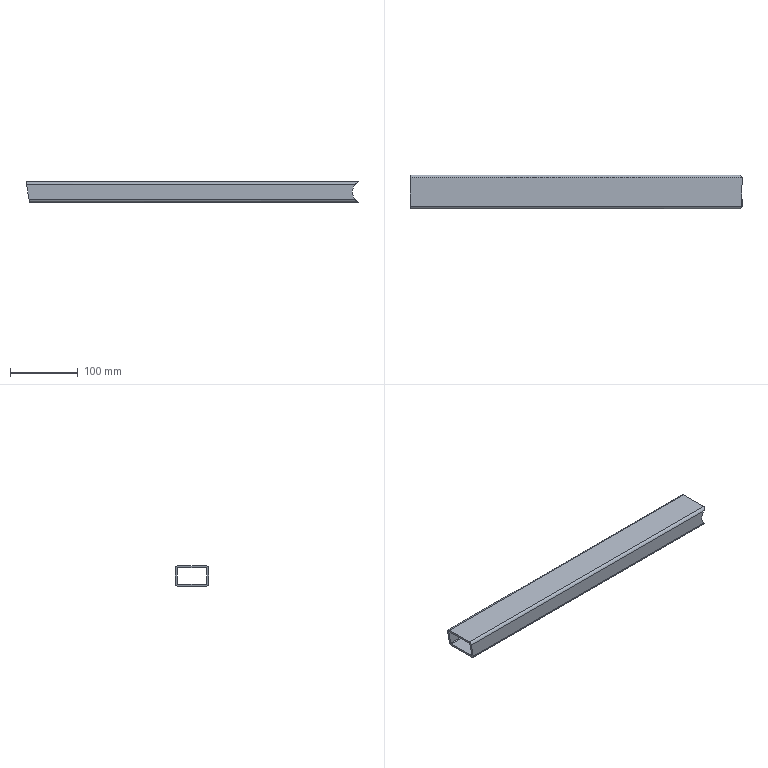Part | SolidWorks | features ICE 2, WeldMemberFeat 1, WeldmentFeature 1 | 1 solid | 18 faces | box 490.986 x 50 x 30 mm | volume 208931 mm3 | cylinder 9 | plane 9 | commonest cylinder face diameters 2 x4 8 x4 35 x1
STEP:
#1=CARTESIAN_POINT('',(-499.295,-25.,11.));
#2=VERTEX_POINT('',#1);
#3=CARTESIAN_POINT('',(-13.611,-25.,11.));
#4=VERTEX_POINT('',#3);
#5=CARTESIAN_POINT('',(-600.,-25.,11.));
#6=DIRECTION('',(1.,0.,0.));
#7=VECTOR('',#6,1000.);
#8=LINE('',#5,#7);
#9=EDGE_CURVE('',#2,#4,#8,.T.);
#10=ORIENTED_EDGE('',*,*,#9,.T.);
#11=CARTESIAN_POINT('',(-9.014,-21.,15.));
#12=VERTEX_POINT('',#11);
#13=CARTESIAN_POINT('',(-13.611,-25.,11.));
#14=CARTESIAN_POINT('',(-13.193,-25.,11.517));
#15=CARTESIAN_POINT('',(-12.756,-24.903,11.998));
#16=CARTESIAN_POINT('',(-11.846,-24.554,12.897));
#17=CARTESIAN_POINT('',(-11.388,-24.308,13.3));
#18=CARTESIAN_POINT('',(-10.713,-23.827,13.84));
#19=CARTESIAN_POINT('',(-10.49,-23.646,14.01));
#20=CARTESIAN_POINT('',(-10.065,-23.248,14.318));
#21=CARTESIAN_POINT('',(-9.861,-23.028,14.459));
#22=CARTESIAN_POINT('',(-9.491,-22.533,14.705));
#23=CARTESIAN_POINT('',(-9.328,-22.264,14.808));
#24=CARTESIAN_POINT('',(-9.146,-21.812,14.92));
#25=CARTESIAN_POINT('',(-9.098,-21.656,14.949));
#26=CARTESIAN_POINT('',(-9.032,-21.335,14.989));
#27=CARTESIAN_POINT('',(-9.014,-21.167,15.));
#28=CARTESIAN_POINT('',(-9.014,-21.,15.));
#29=B_SPLINE_CURVE_WITH_KNOTS('',3,(#13,#14,#15,#16,#17,#18,#19,#20,#21,#22,#23,#24,#25,#26,#27,#28),.UNSPECIFIED.,.F.,.F.,(4,2,2,2,2,2,2,4),(0.,0.001971,0.003942,0.004927,0.005913,0.006898,0.007391,0.007884),.UNSPECIFIED.);
#30=EDGE_CURVE('',#4,#12,#29,.T.);
#31=ORIENTED_EDGE('',*,*,#30,.T.);
#32=CARTESIAN_POINT('',(-500.,-21.,15.));
#33=VERTEX_POINT('',#32);
#34=CARTESIAN_POINT('',(-600.,-21.,15.));
#35=DIRECTION('',(1.,0.,0.));
#36=VECTOR('',#35,1000.);
#37=LINE('',#34,#36);
#38=EDGE_CURVE('',#33,#12,#37,.T.);
#39=ORIENTED_EDGE('',*,*,#38,.F.);
#40=CARTESIAN_POINT('',(-500.,-21.,15.));
#41=CARTESIAN_POINT('',(-500.,-23.343,15.));
#42=CARTESIAN_POINT('',(-499.708,-25.,13.343));
#43=CARTESIAN_POINT('',(-499.295,-25.,11.));
#44=(BOUNDED_CURVE()B_SPLINE_CURVE(3,(#40,#41,#42,#43),.UNSPECIFIED.,.F.,.F.)B_SPLINE_CURVE_WITH_KNOTS((4,4),(3.142,4.712),.UNSPECIFIED.)CURVE()GEOMETRIC_REPRESENTATION_ITEM()RATIONAL_B_SPLINE_CURVE((1.,0.8047,0.8047,1.))REPRESENTATION_ITEM(''));
#45=EDGE_CURVE('',#33,#2,#44,.T.);
#46=ORIENTED_EDGE('',*,*,#45,.T.);
#47=EDGE_LOOP('',(#10,#31,#39,#46));
#48=FACE_OUTER_BOUND('',#47,.T.);
#49=CARTESIAN_POINT('',(-600.,-21.,11.));
#50=DIRECTION('',(1.,0.,0.));
#51=DIRECTION('',(0.,1.,0.));
#52=AXIS2_PLACEMENT_3D('',#49,#50,#51);
#53=CYLINDRICAL_SURFACE('',#52,4.);
#54=ADVANCED_FACE('',(#48),#53,.T.);
#55=ORIENTED_EDGE('',*,*,#38,.T.);
#56=CARTESIAN_POINT('',(-9.014,21.,15.));
#57=VERTEX_POINT('',#56);
#58=CARTESIAN_POINT('',(-9.014,88.,15.));
#59=DIRECTION('',(0.,1.,0.));
#60=VECTOR('',#59,1000.);
#61=LINE('',#58,#60);
#62=EDGE_CURVE('',#12,#57,#61,.T.);
#63=ORIENTED_EDGE('',*,*,#62,.T.);
#64=CARTESIAN_POINT('',(-500.,21.,15.));
#65=VERTEX_POINT('',#64);
#66=CARTESIAN_POINT('',(-600.,21.,15.));
#67=DIRECTION('',(1.,0.,0.));
#68=VECTOR('',#67,1000.);
#69=LINE('',#66,#68);
#70=EDGE_CURVE('',#65,#57,#69,.T.);
#71=ORIENTED_EDGE('',*,*,#70,.F.);
#72=CARTESIAN_POINT('',(-500.,88.,15.));
#73=DIRECTION('',(0.,-1.,0.));
#74=VECTOR('',#73,1000.);
#75=LINE('',#72,#74);
#76=EDGE_CURVE('',#65,#33,#75,.T.);
#77=ORIENTED_EDGE('',*,*,#76,.T.);
#78=EDGE_LOOP('',(#55,#63,#71,#77));
#79=FACE_OUTER_BOUND('',#78,.T.);
#80=CARTESIAN_POINT('',(-600.,-21.,15.));
#81=DIRECTION('',(0.,0.,-1.));
#82=DIRECTION('',(-1.,0.,0.));
#83=AXIS2_PLACEMENT_3D('',#80,#81,#82);
#84=PLANE('',#83);
#85=ADVANCED_FACE('',(#79),#84,.F.);
#86=ORIENTED_EDGE('',*,*,#70,.T.);
#87=CARTESIAN_POINT('',(-13.611,25.,11.));
#88=VERTEX_POINT('',#87);
#89=CARTESIAN_POINT('',(-9.014,21.,15.));
#90=CARTESIAN_POINT('',(-9.014,21.168,15.));
#91=CARTESIAN_POINT('',(-9.031,21.332,14.989));
#92=CARTESIAN_POINT('',(-9.098,21.654,14.949));
#93=CARTESIAN_POINT('',(-9.147,21.813,14.92));
#94=CARTESIAN_POINT('',(-9.267,22.113,14.845));
#95=CARTESIAN_POINT('',(-9.338,22.255,14.801));
#96=CARTESIAN_POINT('',(-9.497,22.528,14.699));
#97=CARTESIAN_POINT('',(-9.585,22.659,14.642));
#98=CARTESIAN_POINT('',(-9.862,23.028,14.459));
#99=CARTESIAN_POINT('',(-10.064,23.247,14.319));
#100=CARTESIAN_POINT('',(-10.49,23.647,14.01));
#101=CARTESIAN_POINT('',(-10.714,23.827,13.84));
#102=CARTESIAN_POINT('',(-11.163,24.147,13.481));
#103=CARTESIAN_POINT('',(-11.389,24.288,13.29));
#104=CARTESIAN_POINT('',(-11.844,24.535,12.887));
#105=CARTESIAN_POINT('',(-12.074,24.642,12.672));
#106=CARTESIAN_POINT('',(-12.755,24.903,11.998));
#107=CARTESIAN_POINT('',(-13.192,25.,11.518));
#108=CARTESIAN_POINT('',(-13.611,25.,11.));
#109=B_SPLINE_CURVE_WITH_KNOTS('',3,(#89,#90,#91,#92,#93,#94,#95,#96,#97,#98,#99,#100,#101,#102,#103,#104,#105,#106,#107,#108),.UNSPECIFIED.,.F.,.F.,(4,2,2,2,2,2,2,2,2,4),(0.,0.0004959,0.0009918,0.001488,0.001984,0.002975,0.003967,0.004959,0.005951,0.007934),.UNSPECIFIED.);
#110=EDGE_CURVE('',#57,#88,#109,.T.);
#111=ORIENTED_EDGE('',*,*,#110,.T.);
#112=CARTESIAN_POINT('',(-499.295,25.,11.));
#113=VERTEX_POINT('',#112);
#114=CARTESIAN_POINT('',(-600.,25.,11.));
#115=DIRECTION('',(1.,0.,0.));
#116=VECTOR('',#115,1000.);
#117=LINE('',#114,#116);
#118=EDGE_CURVE('',#113,#88,#117,.T.);
#119=ORIENTED_EDGE('',*,*,#118,.F.);
#120=CARTESIAN_POINT('',(-499.295,25.,11.));
#121=CARTESIAN_POINT('',(-499.708,25.,13.343));
#122=CARTESIAN_POINT('',(-500.,23.343,15.));
#123=CARTESIAN_POINT('',(-500.,21.,15.));
#124=(BOUNDED_CURVE()B_SPLINE_CURVE(3,(#120,#121,#122,#123),.UNSPECIFIED.,.F.,.F.)B_SPLINE_CURVE_WITH_KNOTS((4,4),(1.571,3.142),.UNSPECIFIED.)CURVE()GEOMETRIC_REPRESENTATION_ITEM()RATIONAL_B_SPLINE_CURVE((1.,0.8047,0.8047,1.))REPRESENTATION_ITEM(''));
#125=EDGE_CURVE('',#113,#65,#124,.T.);
#126=ORIENTED_EDGE('',*,*,#125,.T.);
#127=EDGE_LOOP('',(#86,#111,#119,#126));
#128=FACE_OUTER_BOUND('',#127,.T.);
#129=CARTESIAN_POINT('',(-600.,21.,11.));
#130=DIRECTION('',(1.,0.,0.));
#131=DIRECTION('',(0.,1.,0.));
#132=AXIS2_PLACEMENT_3D('',#129,#130,#131);
#133=CYLINDRICAL_SURFACE('',#132,4.);
#134=ADVANCED_FACE('',(#128),#133,.T.);
#135=ORIENTED_EDGE('',*,*,#118,.T.);
#136=CARTESIAN_POINT('',(-13.611,25.,-11.));
#137=VERTEX_POINT('',#136);
#138=CARTESIAN_POINT('',(0.,25.,0.));
#139=DIRECTION('',(0.,-1.,0.));
#140=DIRECTION('',(1.,0.,0.));
#141=AXIS2_PLACEMENT_3D('',#138,#139,#140);
#142=CIRCLE('',#141,17.5);
#143=EDGE_CURVE('',#88,#137,#142,.T.);
#144=ORIENTED_EDGE('',*,*,#143,.T.);
#145=CARTESIAN_POINT('',(-495.415,25.,-11.));
#146=VERTEX_POINT('',#145);
#147=CARTESIAN_POINT('',(-600.,25.,-11.));
#148=DIRECTION('',(1.,0.,0.));
#149=VECTOR('',#148,1000.);
#150=LINE('',#147,#149);
#151=EDGE_CURVE('',#146,#137,#150,.T.);
#152=ORIENTED_EDGE('',*,*,#151,.F.);
#153=CARTESIAN_POINT('',(-498.569,25.,6.885));
#154=DIRECTION('',(-0.1736,0.,0.9848));
#155=VECTOR('',#154,1000.);
#156=LINE('',#153,#155);
#157=EDGE_CURVE('',#146,#113,#156,.T.);
#158=ORIENTED_EDGE('',*,*,#157,.T.);
#159=EDGE_LOOP('',(#135,#144,#152,#158));
#160=FACE_OUTER_BOUND('',#159,.T.);
#161=CARTESIAN_POINT('',(-600.,25.,-11.));
#162=DIRECTION('',(0.,-1.,0.));
#163=DIRECTION('',(1.,0.,0.));
#164=AXIS2_PLACEMENT_3D('',#161,#162,#163);
#165=PLANE('',#164);
#166=ADVANCED_FACE('',(#160),#165,.F.);
#167=ORIENTED_EDGE('',*,*,#151,.T.);
#168=CARTESIAN_POINT('',(-9.014,21.,-15.));
#169=VERTEX_POINT('',#168);
#170=CARTESIAN_POINT('',(-13.611,25.,-11.));
#171=CARTESIAN_POINT('',(-13.193,25.,-11.517));
#172=CARTESIAN_POINT('',(-12.756,24.903,-11.998));
#173=CARTESIAN_POINT('',(-11.846,24.554,-12.897));
#174=CARTESIAN_POINT('',(-11.388,24.308,-13.3));
#175=CARTESIAN_POINT('',(-10.713,23.827,-13.84));
#176=CARTESIAN_POINT('',(-10.49,23.646,-14.01));
#177=CARTESIAN_POINT('',(-10.065,23.248,-14.318));
#178=CARTESIAN_POINT('',(-9.861,23.028,-14.459));
#179=CARTESIAN_POINT('',(-9.491,22.533,-14.705));
#180=CARTESIAN_POINT('',(-9.328,22.264,-14.808));
#181=CARTESIAN_POINT('',(-9.146,21.812,-14.92));
#182=CARTESIAN_POINT('',(-9.098,21.656,-14.949));
#183=CARTESIAN_POINT('',(-9.032,21.335,-14.989));
#184=CARTESIAN_POINT('',(-9.014,21.167,-15.));
#185=CARTESIAN_POINT('',(-9.014,21.,-15.));
#186=B_SPLINE_CURVE_WITH_KNOTS('',3,(#170,#171,#172,#173,#174,#175,#176,#177,#178,#179,#180,#181,#182,#183,#184,#185),.UNSPECIFIED.,.F.,.F.,(4,2,2,2,2,2,2,4),(0.,0.001971,0.003942,0.004927,0.005913,0.006898,0.007391,0.007884),.UNSPECIFIED.);
#187=EDGE_CURVE('',#137,#169,#186,.T.);
#188=ORIENTED_EDGE('',*,*,#187,.T.);
#189=CARTESIAN_POINT('',(-494.71,21.,-15.));
#190=VERTEX_POINT('',#189);
#191=CARTESIAN_POINT('',(-600.,21.,-15.));
#192=DIRECTION('',(1.,0.,0.));
#193=VECTOR('',#192,1000.);
#194=LINE('',#191,#193);
#195=EDGE_CURVE('',#190,#169,#194,.T.);
#196=ORIENTED_EDGE('',*,*,#195,.F.);
#197=CARTESIAN_POINT('',(-494.71,21.,-15.));
#198=CARTESIAN_POINT('',(-494.71,23.343,-15.));
#199=CARTESIAN_POINT('',(-495.002,25.,-13.343));
#200=CARTESIAN_POINT('',(-495.415,25.,-11.));
#201=(BOUNDED_CURVE()B_SPLINE_CURVE(3,(#197,#198,#199,#200),.UNSPECIFIED.,.F.,.F.)B_SPLINE_CURVE_WITH_KNOTS((4,4),(0.,1.571),.UNSPECIFIED.)CURVE()GEOMETRIC_REPRESENTATION_ITEM()RATIONAL_B_SPLINE_CURVE((1.,0.8047,0.8047,1.))REPRESENTATION_ITEM(''));
#202=EDGE_CURVE('',#190,#146,#201,.T.);
#203=ORIENTED_EDGE('',*,*,#202,.T.);
#204=EDGE_LOOP('',(#167,#188,#196,#203));
#205=FACE_OUTER_BOUND('',#204,.T.);
#206=CARTESIAN_POINT('',(-600.,21.,-11.));
#207=DIRECTION('',(1.,0.,0.));
#208=DIRECTION('',(0.,1.,0.));
#209=AXIS2_PLACEMENT_3D('',#206,#207,#208);
#210=CYLINDRICAL_SURFACE('',#209,4.);
#211=ADVANCED_FACE('',(#205),#210,.T.);
#212=ORIENTED_EDGE('',*,*,#195,.T.);
#213=CARTESIAN_POINT('',(-9.014,-21.,-15.));
#214=VERTEX_POINT('',#213);
#215=CARTESIAN_POINT('',(-9.014,88.,-15.));
#216=DIRECTION('',(0.,-1.,0.));
#217=VECTOR('',#216,1000.);
#218=LINE('',#215,#217);
#219=EDGE_CURVE('',#169,#214,#218,.T.);
#220=ORIENTED_EDGE('',*,*,#219,.T.);
#221=CARTESIAN_POINT('',(-494.71,-21.,-15.));
#222=VERTEX_POINT('',#221);
#223=CARTESIAN_POINT('',(-600.,-21.,-15.));
#224=DIRECTION('',(1.,0.,0.));
#225=VECTOR('',#224,1000.);
#226=LINE('',#223,#225);
#227=EDGE_CURVE('',#222,#214,#226,.T.);
#228=ORIENTED_EDGE('',*,*,#227,.F.);
#229=CARTESIAN_POINT('',(-494.71,88.,-15.));
#230=DIRECTION('',(0.,-1.,0.));
#231=VECTOR('',#230,1000.);
#232=LINE('',#229,#231);
#233=EDGE_CURVE('',#190,#222,#232,.T.);
#234=ORIENTED_EDGE('',*,*,#233,.F.);
#235=EDGE_LOOP('',(#212,#220,#228,#234));
#236=FACE_OUTER_BOUND('',#235,.T.);
#237=CARTESIAN_POINT('',(-600.,21.,-15.));
#238=DIRECTION('',(0.,0.,1.));
#239=DIRECTION('',(1.,0.,0.));
#240=AXIS2_PLACEMENT_3D('',#237,#238,#239);
#241=PLANE('',#240);
#242=ADVANCED_FACE('',(#236),#241,.F.);
#243=ORIENTED_EDGE('',*,*,#227,.T.);
#244=CARTESIAN_POINT('',(-13.611,-25.,-11.));
#245=VERTEX_POINT('',#244);
#246=CARTESIAN_POINT('',(-9.014,-21.,-15.));
#247=CARTESIAN_POINT('',(-9.014,-21.168,-15.));
#248=CARTESIAN_POINT('',(-9.031,-21.332,-14.989));
#249=CARTESIAN_POINT('',(-9.098,-21.654,-14.949));
#250=CARTESIAN_POINT('',(-9.147,-21.813,-14.92));
#251=CARTESIAN_POINT('',(-9.267,-22.113,-14.845));
#252=CARTESIAN_POINT('',(-9.338,-22.255,-14.801));
#253=CARTESIAN_POINT('',(-9.497,-22.528,-14.699));
#254=CARTESIAN_POINT('',(-9.585,-22.659,-14.642));
#255=CARTESIAN_POINT('',(-9.862,-23.028,-14.459));
#256=CARTESIAN_POINT('',(-10.064,-23.247,-14.319));
#257=CARTESIAN_POINT('',(-10.49,-23.647,-14.01));
#258=CARTESIAN_POINT('',(-10.714,-23.827,-13.84));
#259=CARTESIAN_POINT('',(-11.163,-24.147,-13.481));
#260=CARTESIAN_POINT('',(-11.389,-24.288,-13.29));
#261=CARTESIAN_POINT('',(-11.844,-24.535,-12.887));
#262=CARTESIAN_POINT('',(-12.074,-24.642,-12.672));
#263=CARTESIAN_POINT('',(-12.755,-24.903,-11.998));
#264=CARTESIAN_POINT('',(-13.192,-25.,-11.518));
#265=CARTESIAN_POINT('',(-13.611,-25.,-11.));
#266=B_SPLINE_CURVE_WITH_KNOTS('',3,(#246,#247,#248,#249,#250,#251,#252,#253,#254,#255,#256,#257,#258,#259,#260,#261,#262,#263,#264,#265),.UNSPECIFIED.,.F.,.F.,(4,2,2,2,2,2,2,2,2,4),(0.,0.0004959,0.0009918,0.001488,0.001984,0.002975,0.003967,0.004959,0.005951,0.007934),.UNSPECIFIED.);
#267=EDGE_CURVE('',#214,#245,#266,.T.);
#268=ORIENTED_EDGE('',*,*,#267,.T.);
#269=CARTESIAN_POINT('',(-495.415,-25.,-11.));
#270=VERTEX_POINT('',#269);
#271=CARTESIAN_POINT('',(-600.,-25.,-11.));
#272=DIRECTION('',(1.,0.,0.));
#273=VECTOR('',#272,1000.);
#274=LINE('',#271,#273);
#275=EDGE_CURVE('',#270,#245,#274,.T.);
#276=ORIENTED_EDGE('',*,*,#275,.F.);
#277=CARTESIAN_POINT('',(-495.415,-25.,-11.));
#278=CARTESIAN_POINT('',(-495.002,-25.,-13.343));
#279=CARTESIAN_POINT('',(-494.71,-23.343,-15.));
#280=CARTESIAN_POINT('',(-494.71,-21.,-15.));
#281=(BOUNDED_CURVE()B_SPLINE_CURVE(3,(#277,#278,#279,#280),.UNSPECIFIED.,.F.,.F.)B_SPLINE_CURVE_WITH_KNOTS((4,4),(4.712,6.283),.UNSPECIFIED.)CURVE()GEOMETRIC_REPRESENTATION_ITEM()RATIONAL_B_SPLINE_CURVE((1.,0.8047,0.8047,1.))REPRESENTATION_ITEM(''));
#282=EDGE_CURVE('',#270,#222,#281,.T.);
#283=ORIENTED_EDGE('',*,*,#282,.T.);
#284=EDGE_LOOP('',(#243,#268,#276,#283));
#285=FACE_OUTER_BOUND('',#284,.T.);
#286=CARTESIAN_POINT('',(-600.,-21.,-11.));
#287=DIRECTION('',(1.,0.,0.));
#288=DIRECTION('',(0.,1.,0.));
#289=AXIS2_PLACEMENT_3D('',#286,#287,#288);
#290=CYLINDRICAL_SURFACE('',#289,4.);
#291=ADVANCED_FACE('',(#285),#290,.T.);
#292=CARTESIAN_POINT('',(-12.738,21.,12.));
#293=VERTEX_POINT('',#292);
#294=CARTESIAN_POINT('',(-13.611,22.,11.));
#295=VERTEX_POINT('',#294);
#296=CARTESIAN_POINT('',(-12.738,21.,12.));
#297=CARTESIAN_POINT('',(-12.738,21.155,12.));
#298=CARTESIAN_POINT('',(-12.773,21.304,11.963));
#299=CARTESIAN_POINT('',(-12.858,21.496,11.871));
#300=CARTESIAN_POINT('',(-12.892,21.555,11.834));
#301=CARTESIAN_POINT('',(-12.966,21.661,11.753));
#302=CARTESIAN_POINT('',(-13.006,21.708,11.709));
#303=CARTESIAN_POINT('',(-13.134,21.835,11.565));
#304=CARTESIAN_POINT('',(-13.226,21.896,11.46));
#305=CARTESIAN_POINT('',(-13.417,21.979,11.237));
#306=CARTESIAN_POINT('',(-13.514,22.,11.119));
#307=CARTESIAN_POINT('',(-13.611,22.,11.));
#308=B_SPLINE_CURVE_WITH_KNOTS('',3,(#296,#297,#298,#299,#300,#301,#302,#303,#304,#305,#306,#307),.UNSPECIFIED.,.F.,.F.,(4,2,2,2,2,4),(0.,0.0004563,0.0006844,0.0009126,0.001369,0.001825),.UNSPECIFIED.);
#309=EDGE_CURVE('',#293,#295,#308,.T.);
#310=ORIENTED_EDGE('',*,*,#309,.F.);
#311=CARTESIAN_POINT('',(-499.471,21.,12.));
#312=VERTEX_POINT('',#311);
#313=CARTESIAN_POINT('',(-600.,21.,12.));
#314=DIRECTION('',(1.,0.,0.));
#315=VECTOR('',#314,1000.);
#316=LINE('',#313,#315);
#317=EDGE_CURVE('',#312,#293,#316,.T.);
#318=ORIENTED_EDGE('',*,*,#317,.F.);
#319=CARTESIAN_POINT('',(-499.295,22.,11.));
#320=VERTEX_POINT('',#319);
#321=CARTESIAN_POINT('',(-499.295,22.,11.));
#322=CARTESIAN_POINT('',(-499.398,22.,11.586));
#323=CARTESIAN_POINT('',(-499.471,21.586,12.));
#324=CARTESIAN_POINT('',(-499.471,21.,12.));
#325=(BOUNDED_CURVE()B_SPLINE_CURVE(3,(#321,#322,#323,#324),.UNSPECIFIED.,.F.,.F.)B_SPLINE_CURVE_WITH_KNOTS((4,4),(1.571,3.142),.UNSPECIFIED.)CURVE()GEOMETRIC_REPRESENTATION_ITEM()RATIONAL_B_SPLINE_CURVE((1.,0.8047,0.8047,1.))REPRESENTATION_ITEM(''));
#326=EDGE_CURVE('',#320,#312,#325,.T.);
#327=ORIENTED_EDGE('',*,*,#326,.F.);
#328=CARTESIAN_POINT('',(-600.,22.,11.));
#329=DIRECTION('',(1.,0.,0.));
#330=VECTOR('',#329,1000.);
#331=LINE('',#328,#330);
#332=EDGE_CURVE('',#320,#295,#331,.T.);
#333=ORIENTED_EDGE('',*,*,#332,.T.);
#334=EDGE_LOOP('',(#310,#318,#327,#333));
#335=FACE_OUTER_BOUND('',#334,.T.);
#336=CARTESIAN_POINT('',(-600.,21.,11.));
#337=DIRECTION('',(1.,0.,0.));
#338=DIRECTION('',(0.,1.,0.));
#339=AXIS2_PLACEMENT_3D('',#336,#337,#338);
#340=CYLINDRICAL_SURFACE('',#339,1.);
#341=ADVANCED_FACE('',(#335),#340,.F.);
#342=CARTESIAN_POINT('',(-12.738,-21.,12.));
#343=VERTEX_POINT('',#342);
#344=CARTESIAN_POINT('',(-12.738,88.,12.));
#345=DIRECTION('',(0.,1.,0.));
#346=VECTOR('',#345,1000.);
#347=LINE('',#344,#346);
#348=EDGE_CURVE('',#343,#293,#347,.T.);
#349=ORIENTED_EDGE('',*,*,#348,.F.);
#350=CARTESIAN_POINT('',(-499.471,-21.,12.));
#351=VERTEX_POINT('',#350);
#352=CARTESIAN_POINT('',(-600.,-21.,12.));
#353=DIRECTION('',(1.,0.,0.));
#354=VECTOR('',#353,1000.);
#355=LINE('',#352,#354);
#356=EDGE_CURVE('',#351,#343,#355,.T.);
#357=ORIENTED_EDGE('',*,*,#356,.F.);
#358=CARTESIAN_POINT('',(-499.471,-21.,12.));
#359=DIRECTION('',(0.,-1.,0.));
#360=VECTOR('',#359,1000.);
#361=LINE('',#358,#360);
#362=EDGE_CURVE('',#312,#351,#361,.T.);
#363=ORIENTED_EDGE('',*,*,#362,.F.);
#364=ORIENTED_EDGE('',*,*,#317,.T.);
#365=EDGE_LOOP('',(#349,#357,#363,#364));
#366=FACE_OUTER_BOUND('',#365,.T.);
#367=CARTESIAN_POINT('',(-600.,-21.,12.));
#368=DIRECTION('',(0.,0.,-1.));
#369=DIRECTION('',(-1.,0.,0.));
#370=AXIS2_PLACEMENT_3D('',#367,#368,#369);
#371=PLANE('',#370);
#372=ADVANCED_FACE('',(#366),#371,.T.);
#373=CARTESIAN_POINT('',(-13.611,-22.,11.));
#374=VERTEX_POINT('',#373);
#375=CARTESIAN_POINT('',(-13.611,-22.,11.));
#376=CARTESIAN_POINT('',(-13.514,-22.,11.12));
#377=CARTESIAN_POINT('',(-13.418,-21.979,11.235));
#378=CARTESIAN_POINT('',(-13.227,-21.896,11.46));
#379=CARTESIAN_POINT('',(-13.135,-21.835,11.565));
#380=CARTESIAN_POINT('',(-12.966,-21.669,11.754));
#381=CARTESIAN_POINT('',(-12.888,-21.563,11.839));
#382=CARTESIAN_POINT('',(-12.773,-21.305,11.963));
#383=CARTESIAN_POINT('',(-12.738,-21.155,12.));
#384=CARTESIAN_POINT('',(-12.738,-21.,12.));
#385=B_SPLINE_CURVE_WITH_KNOTS('',3,(#375,#376,#377,#378,#379,#380,#381,#382,#383,#384),.UNSPECIFIED.,.F.,.F.,(4,2,2,2,4),(0.,0.0004556,0.0009112,0.001367,0.001822),.UNSPECIFIED.);
#386=EDGE_CURVE('',#374,#343,#385,.T.);
#387=ORIENTED_EDGE('',*,*,#386,.F.);
#388=CARTESIAN_POINT('',(-499.295,-22.,11.));
#389=VERTEX_POINT('',#388);
#390=CARTESIAN_POINT('',(-600.,-22.,11.));
#391=DIRECTION('',(1.,0.,0.));
#392=VECTOR('',#391,1000.);
#393=LINE('',#390,#392);
#394=EDGE_CURVE('',#389,#374,#393,.T.);
#395=ORIENTED_EDGE('',*,*,#394,.F.);
#396=CARTESIAN_POINT('',(-499.471,-21.,12.));
#397=CARTESIAN_POINT('',(-499.471,-21.586,12.));
#398=CARTESIAN_POINT('',(-499.398,-22.,11.586));
#399=CARTESIAN_POINT('',(-499.295,-22.,11.));
#400=(BOUNDED_CURVE()B_SPLINE_CURVE(3,(#396,#397,#398,#399),.UNSPECIFIED.,.F.,.F.)B_SPLINE_CURVE_WITH_KNOTS((4,4),(3.142,4.712),.UNSPECIFIED.)CURVE()GEOMETRIC_REPRESENTATION_ITEM()RATIONAL_B_SPLINE_CURVE((1.,0.8047,0.8047,1.))REPRESENTATION_ITEM(''));
#401=EDGE_CURVE('',#351,#389,#400,.T.);
#402=ORIENTED_EDGE('',*,*,#401,.F.);
#403=ORIENTED_EDGE('',*,*,#356,.T.);
#404=EDGE_LOOP('',(#387,#395,#402,#403));
#405=FACE_OUTER_BOUND('',#404,.T.);
#406=CARTESIAN_POINT('',(-600.,-21.,11.));
#407=DIRECTION('',(1.,0.,0.));
#408=DIRECTION('',(0.,1.,0.));
#409=AXIS2_PLACEMENT_3D('',#406,#407,#408);
#410=CYLINDRICAL_SURFACE('',#409,1.);
#411=ADVANCED_FACE('',(#405),#410,.F.);
#412=CARTESIAN_POINT('',(-13.611,-22.,-11.));
#413=VERTEX_POINT('',#412);
#414=CARTESIAN_POINT('',(0.,-22.,0.));
#415=DIRECTION('',(0.,1.,0.));
#416=DIRECTION('',(-1.,0.,0.));
#417=AXIS2_PLACEMENT_3D('',#414,#415,#416);
#418=CIRCLE('',#417,17.5);
#419=EDGE_CURVE('',#413,#374,#418,.T.);
#420=ORIENTED_EDGE('',*,*,#419,.F.);
#421=CARTESIAN_POINT('',(-495.415,-22.,-11.));
#422=VERTEX_POINT('',#421);
#423=CARTESIAN_POINT('',(-600.,-22.,-11.));
#424=DIRECTION('',(1.,0.,0.));
#425=VECTOR('',#424,1000.);
#426=LINE('',#423,#425);
#427=EDGE_CURVE('',#422,#413,#426,.T.);
#428=ORIENTED_EDGE('',*,*,#427,.F.);
#429=CARTESIAN_POINT('',(-502.331,-22.,28.222));
#430=DIRECTION('',(0.1736,0.,-0.9848));
#431=VECTOR('',#430,1000.);
#432=LINE('',#429,#431);
#433=EDGE_CURVE('',#389,#422,#432,.T.);
#434=ORIENTED_EDGE('',*,*,#433,.F.);
#435=ORIENTED_EDGE('',*,*,#394,.T.);
#436=EDGE_LOOP('',(#420,#428,#434,#435));
#437=FACE_OUTER_BOUND('',#436,.T.);
#438=CARTESIAN_POINT('',(-600.,-22.,11.));
#439=DIRECTION('',(0.,1.,0.));
#440=DIRECTION('',(-1.,0.,0.));
#441=AXIS2_PLACEMENT_3D('',#438,#439,#440);
#442=PLANE('',#441);
#443=ADVANCED_FACE('',(#437),#442,.T.);
#444=CARTESIAN_POINT('',(-12.738,-21.,-12.));
#445=VERTEX_POINT('',#444);
#446=CARTESIAN_POINT('',(-12.738,-21.,-12.));
#447=CARTESIAN_POINT('',(-12.738,-21.155,-12.));
#448=CARTESIAN_POINT('',(-12.773,-21.304,-11.963));
#449=CARTESIAN_POINT('',(-12.858,-21.496,-11.871));
#450=CARTESIAN_POINT('',(-12.892,-21.555,-11.834));
#451=CARTESIAN_POINT('',(-12.966,-21.661,-11.753));
#452=CARTESIAN_POINT('',(-13.006,-21.708,-11.709));
#453=CARTESIAN_POINT('',(-13.134,-21.835,-11.565));
#454=CARTESIAN_POINT('',(-13.226,-21.896,-11.46));
#455=CARTESIAN_POINT('',(-13.417,-21.979,-11.237));
#456=CARTESIAN_POINT('',(-13.514,-22.,-11.119));
#457=CARTESIAN_POINT('',(-13.611,-22.,-11.));
#458=B_SPLINE_CURVE_WITH_KNOTS('',3,(#446,#447,#448,#449,#450,#451,#452,#453,#454,#455,#456,#457),.UNSPECIFIED.,.F.,.F.,(4,2,2,2,2,4),(0.,0.0004563,0.0006844,0.0009126,0.001369,0.001825),.UNSPECIFIED.);
#459=EDGE_CURVE('',#445,#413,#458,.T.);
#460=ORIENTED_EDGE('',*,*,#459,.F.);
#461=CARTESIAN_POINT('',(-495.239,-21.,-12.));
#462=VERTEX_POINT('',#461);
#463=CARTESIAN_POINT('',(-600.,-21.,-12.));
#464=DIRECTION('',(1.,0.,0.));
#465=VECTOR('',#464,1000.);
#466=LINE('',#463,#465);
#467=EDGE_CURVE('',#462,#445,#466,.T.);
#468=ORIENTED_EDGE('',*,*,#467,.F.);
#469=CARTESIAN_POINT('',(-495.415,-22.,-11.));
#470=CARTESIAN_POINT('',(-495.312,-22.,-11.586));
#471=CARTESIAN_POINT('',(-495.239,-21.586,-12.));
#472=CARTESIAN_POINT('',(-495.239,-21.,-12.));
#473=(BOUNDED_CURVE()B_SPLINE_CURVE(3,(#469,#470,#471,#472),.UNSPECIFIED.,.F.,.F.)B_SPLINE_CURVE_WITH_KNOTS((4,4),(4.712,6.283),.UNSPECIFIED.)CURVE()GEOMETRIC_REPRESENTATION_ITEM()RATIONAL_B_SPLINE_CURVE((1.,0.8047,0.8047,1.))REPRESENTATION_ITEM(''));
#474=EDGE_CURVE('',#422,#462,#473,.T.);
#475=ORIENTED_EDGE('',*,*,#474,.F.);
#476=ORIENTED_EDGE('',*,*,#427,.T.);
#477=EDGE_LOOP('',(#460,#468,#475,#476));
#478=FACE_OUTER_BOUND('',#477,.T.);
#479=CARTESIAN_POINT('',(-600.,-21.,-11.));
#480=DIRECTION('',(1.,0.,0.));
#481=DIRECTION('',(0.,1.,0.));
#482=AXIS2_PLACEMENT_3D('',#479,#480,#481);
#483=CYLINDRICAL_SURFACE('',#482,1.);
#484=ADVANCED_FACE('',(#478),#483,.F.);
#485=CARTESIAN_POINT('',(-12.738,21.,-12.));
#486=VERTEX_POINT('',#485);
#487=CARTESIAN_POINT('',(-12.738,88.,-12.));
#488=DIRECTION('',(0.,-1.,0.));
#489=VECTOR('',#488,1000.);
#490=LINE('',#487,#489);
#491=EDGE_CURVE('',#486,#445,#490,.T.);
#492=ORIENTED_EDGE('',*,*,#491,.F.);
#493=CARTESIAN_POINT('',(-495.239,21.,-12.));
#494=VERTEX_POINT('',#493);
#495=CARTESIAN_POINT('',(-600.,21.,-12.));
#496=DIRECTION('',(1.,0.,0.));
#497=VECTOR('',#496,1000.);
#498=LINE('',#495,#497);
#499=EDGE_CURVE('',#494,#486,#498,.T.);
#500=ORIENTED_EDGE('',*,*,#499,.F.);
#501=CARTESIAN_POINT('',(-495.239,21.,-12.));
#502=DIRECTION('',(0.,1.,0.));
#503=VECTOR('',#502,1000.);
#504=LINE('',#501,#503);
#505=EDGE_CURVE('',#462,#494,#504,.T.);
#506=ORIENTED_EDGE('',*,*,#505,.F.);
#507=ORIENTED_EDGE('',*,*,#467,.T.);
#508=EDGE_LOOP('',(#492,#500,#506,#507));
#509=FACE_OUTER_BOUND('',#508,.T.);
#510=CARTESIAN_POINT('',(-600.,21.,-12.));
#511=DIRECTION('',(0.,0.,1.));
#512=DIRECTION('',(1.,0.,0.));
#513=AXIS2_PLACEMENT_3D('',#510,#511,#512);
#514=PLANE('',#513);
#515=ADVANCED_FACE('',(#509),#514,.T.);
#516=CARTESIAN_POINT('',(-13.611,22.,-11.));
#517=VERTEX_POINT('',#516);
#518=CARTESIAN_POINT('',(-13.611,22.,-11.));
#519=CARTESIAN_POINT('',(-13.514,22.,-11.12));
#520=CARTESIAN_POINT('',(-13.418,21.979,-11.235));
#521=CARTESIAN_POINT('',(-13.227,21.896,-11.46));
#522=CARTESIAN_POINT('',(-13.135,21.835,-11.565));
#523=CARTESIAN_POINT('',(-12.966,21.669,-11.754));
#524=CARTESIAN_POINT('',(-12.888,21.563,-11.839));
#525=CARTESIAN_POINT('',(-12.773,21.305,-11.963));
#526=CARTESIAN_POINT('',(-12.738,21.155,-12.));
#527=CARTESIAN_POINT('',(-12.738,21.,-12.));
#528=B_SPLINE_CURVE_WITH_KNOTS('',3,(#518,#519,#520,#521,#522,#523,#524,#525,#526,#527),.UNSPECIFIED.,.F.,.F.,(4,2,2,2,4),(0.,0.0004556,0.0009112,0.001367,0.001822),.UNSPECIFIED.);
#529=EDGE_CURVE('',#517,#486,#528,.T.);
#530=ORIENTED_EDGE('',*,*,#529,.F.);
#531=CARTESIAN_POINT('',(-495.415,22.,-11.));
#532=VERTEX_POINT('',#531);
#533=CARTESIAN_POINT('',(-600.,22.,-11.));
#534=DIRECTION('',(1.,0.,0.));
#535=VECTOR('',#534,1000.);
#536=LINE('',#533,#535);
#537=EDGE_CURVE('',#532,#517,#536,.T.);
#538=ORIENTED_EDGE('',*,*,#537,.F.);
#539=CARTESIAN_POINT('',(-495.239,21.,-12.));
#540=CARTESIAN_POINT('',(-495.239,21.586,-12.));
#541=CARTESIAN_POINT('',(-495.312,22.,-11.586));
#542=CARTESIAN_POINT('',(-495.415,22.,-11.));
#543=(BOUNDED_CURVE()B_SPLINE_CURVE(3,(#539,#540,#541,#542),.UNSPECIFIED.,.F.,.T.)B_SPLINE_CURVE_WITH_KNOTS((4,4),(0.,1.571),.UNSPECIFIED.)CURVE()GEOMETRIC_REPRESENTATION_ITEM()RATIONAL_B_SPLINE_CURVE((1.,0.8047,0.8047,1.))REPRESENTATION_ITEM(''));
#544=EDGE_CURVE('',#494,#532,#543,.T.);
#545=ORIENTED_EDGE('',*,*,#544,.F.);
#546=ORIENTED_EDGE('',*,*,#499,.T.);
#547=EDGE_LOOP('',(#530,#538,#545,#546));
#548=FACE_OUTER_BOUND('',#547,.T.);
#549=CARTESIAN_POINT('',(-600.,21.,-11.));
#550=DIRECTION('',(1.,0.,0.));
#551=DIRECTION('',(0.,1.,0.));
#552=AXIS2_PLACEMENT_3D('',#549,#550,#551);
#553=CYLINDRICAL_SURFACE('',#552,1.);
#554=ADVANCED_FACE('',(#548),#553,.F.);
#555=CARTESIAN_POINT('',(0.,22.,0.));
#556=DIRECTION('',(0.,-1.,0.));
#557=DIRECTION('',(1.,0.,0.));
#558=AXIS2_PLACEMENT_3D('',#555,#556,#557);
#559=CIRCLE('',#558,17.5);
#560=EDGE_CURVE('',#295,#517,#559,.T.);
#561=ORIENTED_EDGE('',*,*,#560,.F.);
#562=ORIENTED_EDGE('',*,*,#332,.F.);
#563=CARTESIAN_POINT('',(-498.569,22.,6.885));
#564=DIRECTION('',(-0.1736,0.,0.9848));
#565=VECTOR('',#564,1000.);
#566=LINE('',#563,#565);
#567=EDGE_CURVE('',#532,#320,#566,.T.);
#568=ORIENTED_EDGE('',*,*,#567,.F.);
#569=ORIENTED_EDGE('',*,*,#537,.T.);
#570=EDGE_LOOP('',(#561,#562,#568,#569));
#571=FACE_OUTER_BOUND('',#570,.T.);
#572=CARTESIAN_POINT('',(-600.,22.,-11.));
#573=DIRECTION('',(0.,-1.,0.));
#574=DIRECTION('',(1.,0.,0.));
#575=AXIS2_PLACEMENT_3D('',#572,#573,#574);
#576=PLANE('',#575);
#577=ADVANCED_FACE('',(#571),#576,.T.);
#578=ORIENTED_EDGE('',*,*,#275,.T.);
#579=CARTESIAN_POINT('',(0.,-25.,0.));
#580=DIRECTION('',(0.,-1.,0.));
#581=DIRECTION('',(1.,0.,0.));
#582=AXIS2_PLACEMENT_3D('',#579,#580,#581);
#583=CIRCLE('',#582,17.5);
#584=EDGE_CURVE('',#4,#245,#583,.T.);
#585=ORIENTED_EDGE('',*,*,#584,.F.);
#586=ORIENTED_EDGE('',*,*,#9,.F.);
#587=CARTESIAN_POINT('',(-500.,-25.,15.));
#588=DIRECTION('',(-0.1736,0.,0.9848));
#589=VECTOR('',#588,1000.);
#590=LINE('',#587,#589);
#591=EDGE_CURVE('',#270,#2,#590,.T.);
#592=ORIENTED_EDGE('',*,*,#591,.F.);
#593=EDGE_LOOP('',(#578,#585,#586,#592));
#594=FACE_OUTER_BOUND('',#593,.T.);
#595=CARTESIAN_POINT('',(-600.,-25.,11.));
#596=DIRECTION('',(0.,1.,0.));
#597=DIRECTION('',(-1.,0.,0.));
#598=AXIS2_PLACEMENT_3D('',#595,#596,#597);
#599=PLANE('',#598);
#600=ADVANCED_FACE('',(#594),#599,.F.);
#601=ORIENTED_EDGE('',*,*,#326,.T.);
#602=ORIENTED_EDGE('',*,*,#362,.T.);
#603=ORIENTED_EDGE('',*,*,#401,.T.);
#604=ORIENTED_EDGE('',*,*,#433,.T.);
#605=ORIENTED_EDGE('',*,*,#474,.T.);
#606=ORIENTED_EDGE('',*,*,#505,.T.);
#607=ORIENTED_EDGE('',*,*,#544,.T.);
#608=ORIENTED_EDGE('',*,*,#567,.T.);
#609=EDGE_LOOP('',(#601,#602,#603,#604,#605,#606,#607,#608));
#610=FACE_BOUND('',#609,.T.);
#611=ORIENTED_EDGE('',*,*,#76,.F.);
#612=ORIENTED_EDGE('',*,*,#125,.F.);
#613=ORIENTED_EDGE('',*,*,#157,.F.);
#614=ORIENTED_EDGE('',*,*,#202,.F.);
#615=ORIENTED_EDGE('',*,*,#233,.T.);
#616=ORIENTED_EDGE('',*,*,#282,.F.);
#617=ORIENTED_EDGE('',*,*,#591,.T.);
#618=ORIENTED_EDGE('',*,*,#45,.F.);
#619=EDGE_LOOP('',(#611,#612,#613,#614,#615,#616,#617,#618));
#620=FACE_OUTER_BOUND('',#619,.T.);
#621=CARTESIAN_POINT('',(-500.,88.,15.));
#622=DIRECTION('',(0.9848,0.,0.1736));
#623=DIRECTION('',(0.1736,0.,-0.9848));
#624=AXIS2_PLACEMENT_3D('',#621,#622,#623);
#625=PLANE('',#624);
#626=ADVANCED_FACE('',(#610,#620),#625,.F.);
#627=ORIENTED_EDGE('',*,*,#309,.T.);
#628=ORIENTED_EDGE('',*,*,#560,.T.);
#629=ORIENTED_EDGE('',*,*,#529,.T.);
#630=ORIENTED_EDGE('',*,*,#491,.T.);
#631=ORIENTED_EDGE('',*,*,#459,.T.);
#632=ORIENTED_EDGE('',*,*,#419,.T.);
#633=ORIENTED_EDGE('',*,*,#386,.T.);
#634=ORIENTED_EDGE('',*,*,#348,.T.);
#635=EDGE_LOOP('',(#627,#628,#629,#630,#631,#632,#633,#634));
#636=FACE_BOUND('',#635,.T.);
#637=ORIENTED_EDGE('',*,*,#584,.T.);
#638=ORIENTED_EDGE('',*,*,#267,.F.);
#639=ORIENTED_EDGE('',*,*,#219,.F.);
#640=ORIENTED_EDGE('',*,*,#187,.F.);
#641=ORIENTED_EDGE('',*,*,#143,.F.);
#642=ORIENTED_EDGE('',*,*,#110,.F.);
#643=ORIENTED_EDGE('',*,*,#62,.F.);
#644=ORIENTED_EDGE('',*,*,#30,.F.);
#645=EDGE_LOOP('',(#637,#638,#639,#640,#641,#642,#643,#644));
#646=FACE_OUTER_BOUND('',#645,.T.);
#647=CARTESIAN_POINT('',(0.,88.,0.));
#648=DIRECTION('',(0.,-1.,0.));
#649=DIRECTION('',(1.,0.,0.));
#650=AXIS2_PLACEMENT_3D('',#647,#648,#649);
#651=CYLINDRICAL_SURFACE('',#650,17.5);
#652=ADVANCED_FACE('',(#636,#646),#651,.F.);
#653=CLOSED_SHELL('',(#54,#85,#134,#166,#211,#242,#291,#341,#372,#411,#443,#484,#515,#554,#577,#600,#626,#652));
#654=MANIFOLD_SOLID_BREP('',#653);
#655=CARTESIAN_POINT('',(0.,0.,0.));
#656=DIRECTION('',(0.,0.,1.));
#657=DIRECTION('',(1.,0.,0.));
#658=AXIS2_PLACEMENT_3D('',#655,#656,#657);
#659=(LENGTH_UNIT()NAMED_UNIT(*)SI_UNIT(.MILLI.,.METRE.));
#660=UNCERTAINTY_MEASURE_WITH_UNIT(LENGTH_MEASURE(0.00001),#659,'','');
#661=(NAMED_UNIT(*)PLANE_ANGLE_UNIT()SI_UNIT($,.RADIAN.));
#662=(NAMED_UNIT(*)SI_UNIT($,.STERADIAN.)SOLID_ANGLE_UNIT());
#663=(GEOMETRIC_REPRESENTATION_CONTEXT(3)GLOBAL_UNCERTAINTY_ASSIGNED_CONTEXT((#660))GLOBAL_UNIT_ASSIGNED_CONTEXT((#659,#661,#662))REPRESENTATION_CONTEXT('',''));
#664=ADVANCED_BREP_SHAPE_REPRESENTATION('',(#654,#658),#663);